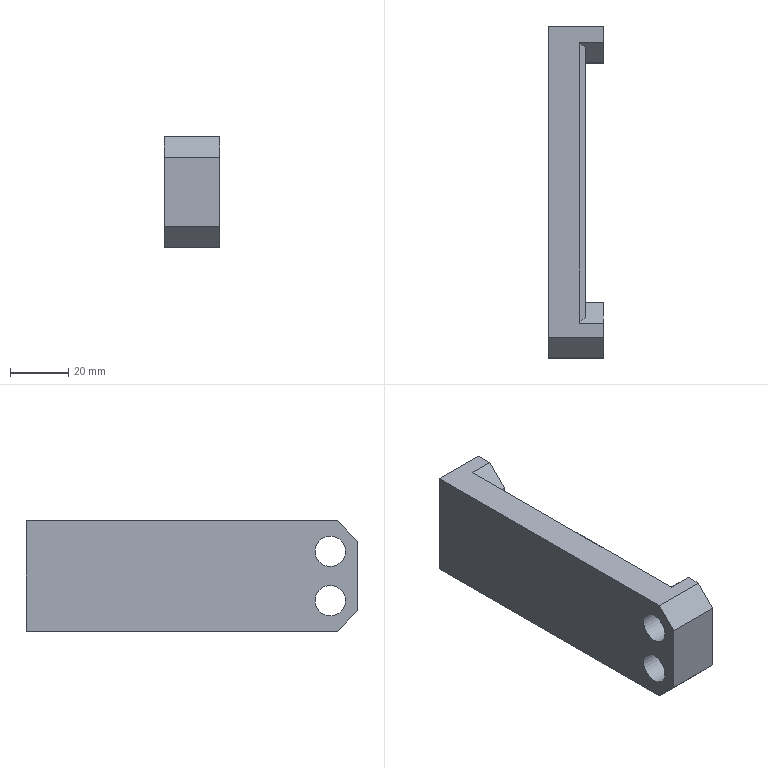Part | STEP file | 1_id1546_x_t | 1 solid | 20 faces | box 19.05 x 114.3 x 38.1 mm | volume 57701 mm3 | plane 18 | cylinder 2 | commonest cylinder face diameters 10.5 x2